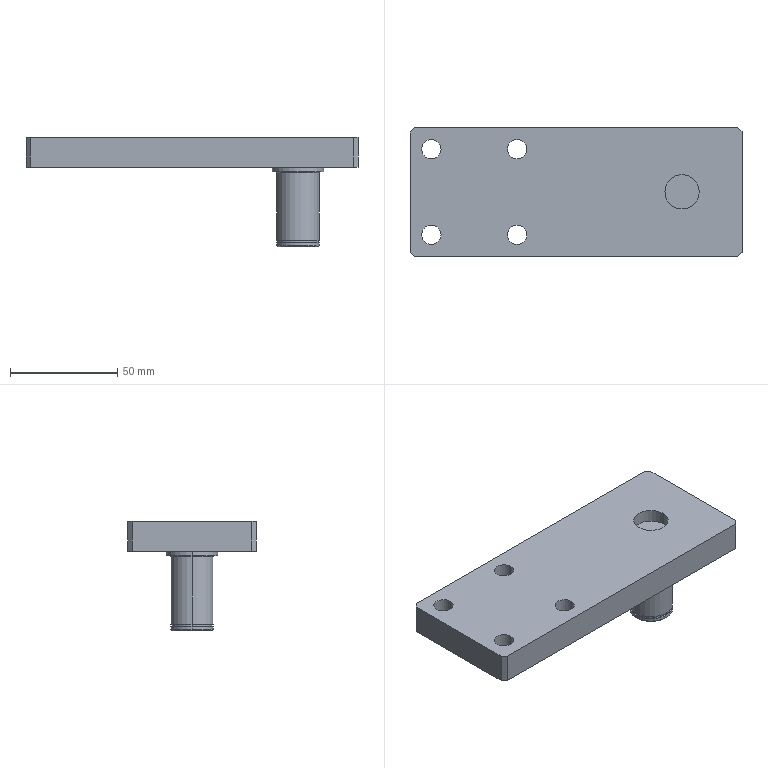Part | SolidWorks | features BaseBody 2 | 2 solids | 68 faces | box 155 x 60 x 51 mm | volume 133278 mm3 | cylinder 36 | plane 20 | cone 10 | spline 2 | commonest cylinder face diameters 3.3 x8 9 x8 15 x8 16 x4 20 x4 19 x2